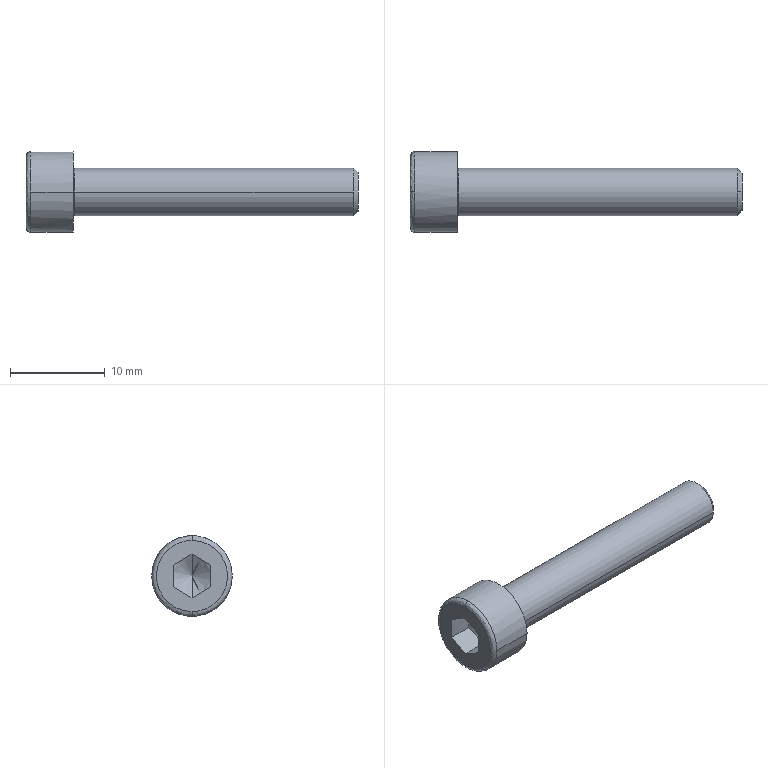Part | STEP file | AS 1420 - Metric M5 x 30 | 1 solid | 21 faces | box 35 x 8.5 x 8.5 mm | volume 827.769 mm3 | plane 9 | spline 4 | cylinder 4 | cone 4 | commonest cylinder face diameters 5 x2 8.5 x2